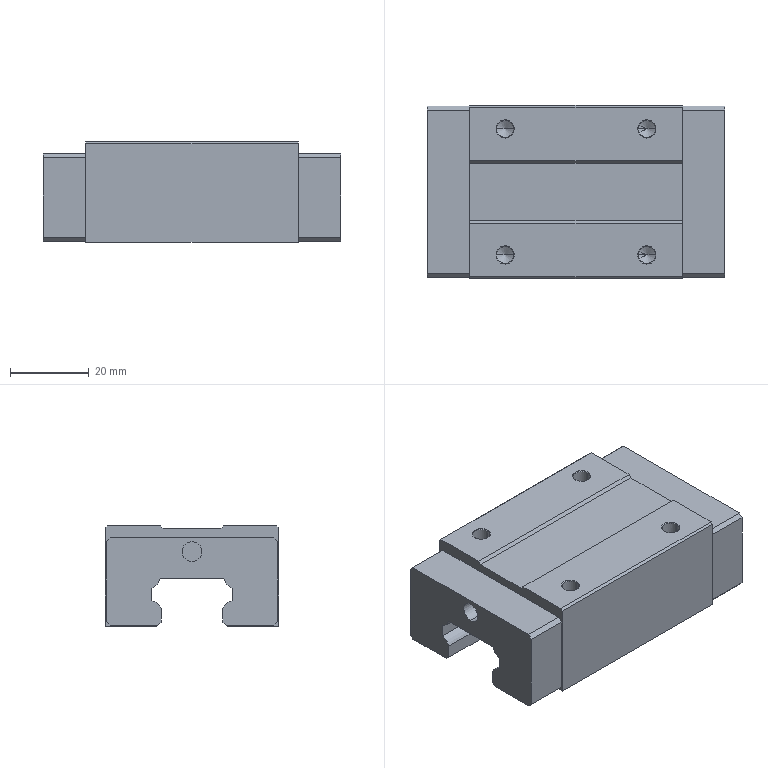Part | SolidWorks | features BaseBody 1 | 1 solid | 90 faces | box 75.6 x 44 x 25.4 mm | volume 63820 mm3 | plane 54 | cylinder 20 | cone 16 | commonest cylinder face diameters 4.3 x8 7.4 x8 5 x4